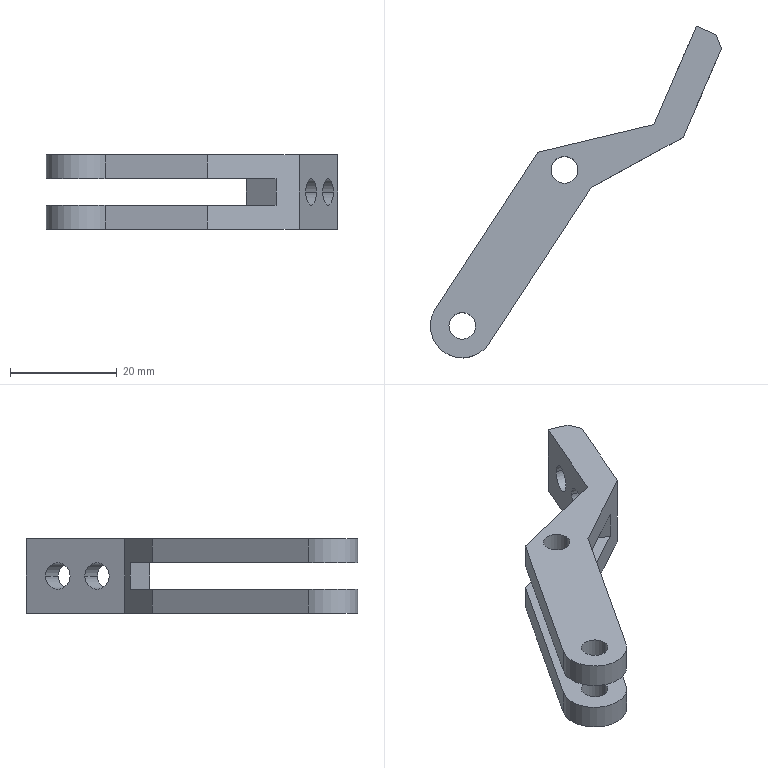Part | STEP file | gripper arm 4_default | 1 solid | 29 faces | box 54.647 x 62.275 x 14 mm | volume 6777 mm3 | plane 15 | cylinder 14 | commonest cylinder face diameters 5 x12 12 x2